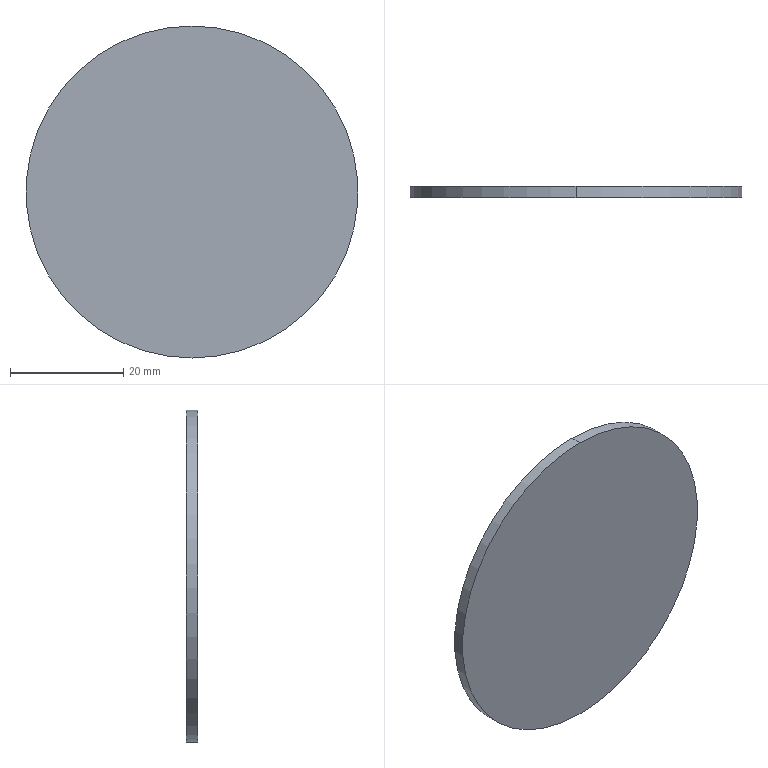Part | SolidWorks | features RefAxis 9, 3DProfileFeature 3, Revolution 1 | 1 solid | 4 faces | box 58.511 x 2 x 58.511 mm | volume 5378 mm3 | cylinder 2 | plane 2 | commonest cylinder face diameters 58.511 x2
STEP:
#1=CARTESIAN_POINT('',(0.,-16.2,29.256));
#2=VERTEX_POINT('',#1);
#3=CARTESIAN_POINT('',(0.,-16.2,-29.256));
#4=VERTEX_POINT('',#3);
#5=CARTESIAN_POINT('',(0.,-16.2,0.));
#6=DIRECTION('',(0.,1.,0.));
#7=DIRECTION('',(0.,0.,1.));
#8=AXIS2_PLACEMENT_3D('',#5,#6,#7);
#9=CIRCLE('',#8,29.256);
#10=EDGE_CURVE('',#2,#4,#9,.T.);
#11=ORIENTED_EDGE('',*,*,#10,.T.);
#12=CARTESIAN_POINT('',(0.,-14.2,-29.256));
#13=VERTEX_POINT('',#12);
#14=CARTESIAN_POINT('',(0.,-14.2,-29.256));
#15=DIRECTION('',(0.,1.,0.));
#16=VECTOR('',#15,1000.);
#17=LINE('',#14,#16);
#18=EDGE_CURVE('',#4,#13,#17,.T.);
#19=ORIENTED_EDGE('',*,*,#18,.T.);
#20=CARTESIAN_POINT('',(0.,-14.2,29.256));
#21=VERTEX_POINT('',#20);
#22=CARTESIAN_POINT('',(0.,-14.2,0.));
#23=DIRECTION('',(0.,1.,0.));
#24=DIRECTION('',(0.,0.,1.));
#25=AXIS2_PLACEMENT_3D('',#22,#23,#24);
#26=CIRCLE('',#25,29.256);
#27=EDGE_CURVE('',#21,#13,#26,.T.);
#28=ORIENTED_EDGE('',*,*,#27,.F.);
#29=CARTESIAN_POINT('',(0.,-14.2,29.256));
#30=DIRECTION('',(0.,1.,0.));
#31=VECTOR('',#30,1000.);
#32=LINE('',#29,#31);
#33=EDGE_CURVE('',#2,#21,#32,.T.);
#34=ORIENTED_EDGE('',*,*,#33,.F.);
#35=EDGE_LOOP('',(#11,#19,#28,#34));
#36=FACE_OUTER_BOUND('',#35,.T.);
#37=CARTESIAN_POINT('',(0.,-14.2,0.));
#38=DIRECTION('',(0.,1.,0.));
#39=DIRECTION('',(0.,0.,1.));
#40=AXIS2_PLACEMENT_3D('',#37,#38,#39);
#41=CYLINDRICAL_SURFACE('',#40,29.256);
#42=ADVANCED_FACE('',(#36),#41,.T.);
#43=ORIENTED_EDGE('',*,*,#27,.T.);
#44=CARTESIAN_POINT('',(0.,-14.2,0.));
#45=DIRECTION('',(0.,1.,0.));
#46=DIRECTION('',(0.,0.,1.));
#47=AXIS2_PLACEMENT_3D('',#44,#45,#46);
#48=CIRCLE('',#47,29.256);
#49=EDGE_CURVE('',#13,#21,#48,.T.);
#50=ORIENTED_EDGE('',*,*,#49,.T.);
#51=EDGE_LOOP('',(#43,#50));
#52=FACE_OUTER_BOUND('',#51,.T.);
#53=CARTESIAN_POINT('',(0.,-14.2,0.));
#54=DIRECTION('',(0.,-1.,0.));
#55=DIRECTION('',(0.,0.,-1.));
#56=AXIS2_PLACEMENT_3D('',#53,#54,#55);
#57=PLANE('',#56);
#58=ADVANCED_FACE('',(#52),#57,.F.);
#59=ORIENTED_EDGE('',*,*,#18,.F.);
#60=CARTESIAN_POINT('',(0.,-16.2,0.));
#61=DIRECTION('',(0.,1.,0.));
#62=DIRECTION('',(0.,0.,1.));
#63=AXIS2_PLACEMENT_3D('',#60,#61,#62);
#64=CIRCLE('',#63,29.256);
#65=EDGE_CURVE('',#4,#2,#64,.T.);
#66=ORIENTED_EDGE('',*,*,#65,.T.);
#67=ORIENTED_EDGE('',*,*,#33,.T.);
#68=ORIENTED_EDGE('',*,*,#49,.F.);
#69=EDGE_LOOP('',(#59,#66,#67,#68));
#70=FACE_OUTER_BOUND('',#69,.T.);
#71=CARTESIAN_POINT('',(0.,-14.2,0.));
#72=DIRECTION('',(0.,1.,0.));
#73=DIRECTION('',(0.,0.,1.));
#74=AXIS2_PLACEMENT_3D('',#71,#72,#73);
#75=CYLINDRICAL_SURFACE('',#74,29.256);
#76=ADVANCED_FACE('',(#70),#75,.T.);
#77=ORIENTED_EDGE('',*,*,#10,.F.);
#78=ORIENTED_EDGE('',*,*,#65,.F.);
#79=EDGE_LOOP('',(#77,#78));
#80=FACE_OUTER_BOUND('',#79,.T.);
#81=CARTESIAN_POINT('',(29.256,-16.2,0.));
#82=DIRECTION('',(0.,1.,0.));
#83=DIRECTION('',(0.,0.,1.));
#84=AXIS2_PLACEMENT_3D('',#81,#82,#83);
#85=PLANE('',#84);
#86=ADVANCED_FACE('',(#80),#85,.F.);
#87=CLOSED_SHELL('',(#42,#58,#76,#86));
#88=MANIFOLD_SOLID_BREP('',#87);
#89=CARTESIAN_POINT('',(0.,0.,0.));
#90=DIRECTION('',(0.,0.,1.));
#91=DIRECTION('',(1.,0.,0.));
#92=AXIS2_PLACEMENT_3D('',#89,#90,#91);
#93=(LENGTH_UNIT()NAMED_UNIT(*)SI_UNIT(.MILLI.,.METRE.));
#94=UNCERTAINTY_MEASURE_WITH_UNIT(LENGTH_MEASURE(0.00001),#93,'','');
#95=(NAMED_UNIT(*)PLANE_ANGLE_UNIT()SI_UNIT($,.RADIAN.));
#96=(NAMED_UNIT(*)SI_UNIT($,.STERADIAN.)SOLID_ANGLE_UNIT());
#97=(GEOMETRIC_REPRESENTATION_CONTEXT(3)GLOBAL_UNCERTAINTY_ASSIGNED_CONTEXT((#94))GLOBAL_UNIT_ASSIGNED_CONTEXT((#93,#95,#96))REPRESENTATION_CONTEXT('',''));
#98=ADVANCED_BREP_SHAPE_REPRESENTATION('',(#88,#92),#97);